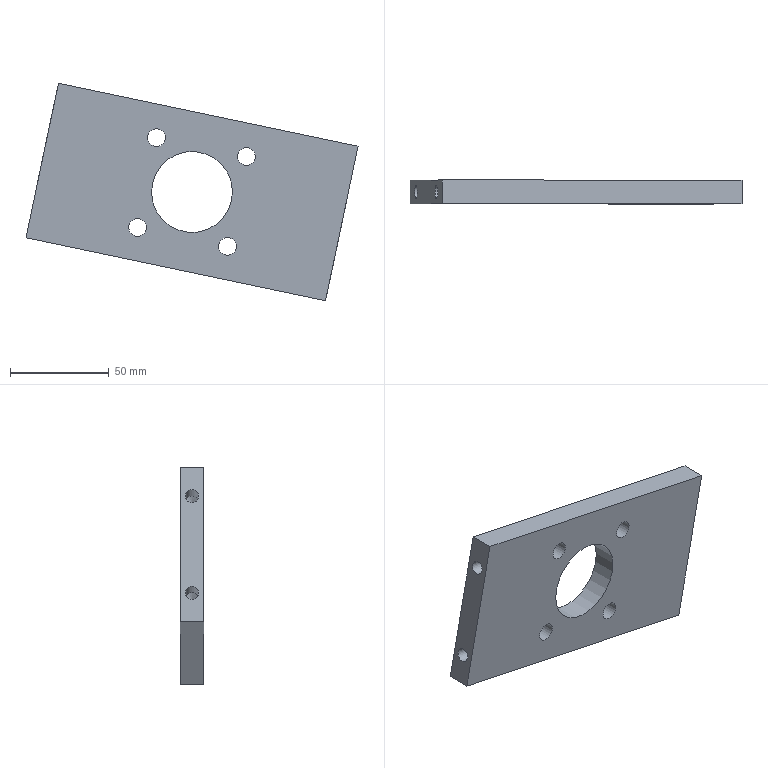Part | STEP file | SN10_007_005_PLACA | 1 solid | 19 faces | box 168.139 x 12 x 110.165 mm | volume 127729 mm3 | cylinder 9 | plane 6 | cone 4 | commonest cylinder face diameters 6.647 x4 9 x4 41 x1
STEP:
#1=CARTESIAN_POINT('',(0.,0.,0.));
#2=DIRECTION('',(0.,0.,1.));
#3=DIRECTION('',(1.,0.,0.));
#4=AXIS2_PLACEMENT_3D('',#1,#2,#3);
#5=CARTESIAN_POINT('',(-580.508,-921.15,530.345));
#6=VERTEX_POINT('',#5);
#7=CARTESIAN_POINT('',(-600.57,-921.15,534.561));
#8=DIRECTION('',(0.,1.,0.));
#9=DIRECTION('',(-0.9786,0.,0.2056));
#10=AXIS2_PLACEMENT_3D('',#7,#8,#9);
#11=CIRCLE('',#10,20.5);
#12=CARTESIAN_POINT('',(-600.57,-909.15,534.561));
#13=DIRECTION('',(0.,-1.,0.));
#14=DIRECTION('',(-0.9786,0.,0.2056));
#15=AXIS2_PLACEMENT_3D('',#12,#13,#14);
#16=CYLINDRICAL_SURFACE('',#15,20.5);
#17=CARTESIAN_POINT('',(12.566,12.));
#18=DIRECTION('',(-1.,0.));
#19=VECTOR('',#18,1.);
#20=LINE('',#17,#19);
#21=(GEOMETRIC_REPRESENTATION_CONTEXT(2)PARAMETRIC_REPRESENTATION_CONTEXT()REPRESENTATION_CONTEXT('',''));
#22=DEFINITIONAL_REPRESENTATION('',(#20),#21);
#23=PCURVE('',#16,#22);
#24=CARTESIAN_POINT('',(-537.207,-921.15,495.7));
#25=DIRECTION('',(0.,-1.,0.));
#26=DIRECTION('',(0.,0.,-1.));
#27=AXIS2_PLACEMENT_3D('',#24,#25,#26);
#28=PLANE('',#27);
#29=CARTESIAN_POINT('',(-43.076,-83.425));
#30=CARTESIAN_POINT('',(-77.825,-76.123));
#31=CARTESIAN_POINT('',(-54.127,-49.681));
#32=CARTESIAN_POINT('',(-30.429,-23.239));
#33=CARTESIAN_POINT('',(-19.379,-56.983));
#34=CARTESIAN_POINT('',(-8.328,-90.726));
#35=CARTESIAN_POINT('',(-43.076,-83.425));
#36=(BOUNDED_CURVE()B_SPLINE_CURVE(2,(#29,#30,#31,#32,#33,#34,#35),.UNSPECIFIED.,.T.,.F.)B_SPLINE_CURVE_WITH_KNOTS((1,2,2,2,2,1),(-2.094,0.,2.094,4.189,6.283,8.378),.UNSPECIFIED.)CURVE()GEOMETRIC_REPRESENTATION_ITEM()RATIONAL_B_SPLINE_CURVE((1.,0.5,1.,0.5,1.,0.5,1.))REPRESENTATION_ITEM(''));
#37=(GEOMETRIC_REPRESENTATION_CONTEXT(2)PARAMETRIC_REPRESENTATION_CONTEXT()REPRESENTATION_CONTEXT('',''));
#38=DEFINITIONAL_REPRESENTATION('',(#36),#37);
#39=PCURVE('',#28,#38);
#40=SURFACE_CURVE('',#11,(#23,#39),.PCURVE_S1.);
#41=EDGE_CURVE('',#6,#6,#40,.T.);
#42=ORIENTED_EDGE('',*,*,#41,.T.);
#43=CARTESIAN_POINT('',(-580.508,-909.15,530.345));
#44=VERTEX_POINT('',#43);
#45=CARTESIAN_POINT('',(-580.508,-909.15,530.345));
#46=CARTESIAN_POINT('',(-580.508,-921.15,530.345));
#47=B_SPLINE_CURVE_WITH_KNOTS('',1,(#45,#46),.UNSPECIFIED.,.F.,.F.,(2,2),(0.,12.),.PIECEWISE_BEZIER_KNOTS.);
#48=CARTESIAN_POINT('',(3.142,0.));
#49=DIRECTION('',(0.,1.));
#50=VECTOR('',#49,1.);
#51=LINE('',#48,#50);
#52=(GEOMETRIC_REPRESENTATION_CONTEXT(2)PARAMETRIC_REPRESENTATION_CONTEXT()REPRESENTATION_CONTEXT('',''));
#53=DEFINITIONAL_REPRESENTATION('',(#51),#52);
#54=PCURVE('',#16,#53);
#55=CARTESIAN_POINT('',(9.425,0.));
#56=DIRECTION('',(0.,1.));
#57=VECTOR('',#56,1.);
#58=LINE('',#55,#57);
#59=(GEOMETRIC_REPRESENTATION_CONTEXT(2)PARAMETRIC_REPRESENTATION_CONTEXT()REPRESENTATION_CONTEXT('',''));
#60=DEFINITIONAL_REPRESENTATION('',(#58),#59);
#61=PCURVE('',#16,#60);
#62=SEAM_CURVE('',#47,(#54,#61),.PCURVE_S1.);
#63=EDGE_CURVE('',#44,#6,#62,.T.);
#64=ORIENTED_EDGE('',*,*,#63,.F.);
#65=CARTESIAN_POINT('',(-600.57,-909.15,534.561));
#66=DIRECTION('',(0.,-1.,0.));
#67=DIRECTION('',(-0.9786,0.,0.2056));
#68=AXIS2_PLACEMENT_3D('',#65,#66,#67);
#69=CIRCLE('',#68,20.5);
#70=CARTESIAN_POINT('',(0.,0.));
#71=DIRECTION('',(1.,0.));
#72=VECTOR('',#71,1.);
#73=LINE('',#70,#72);
#74=(GEOMETRIC_REPRESENTATION_CONTEXT(2)PARAMETRIC_REPRESENTATION_CONTEXT()REPRESENTATION_CONTEXT('',''));
#75=DEFINITIONAL_REPRESENTATION('',(#73),#74);
#76=PCURVE('',#16,#75);
#77=CARTESIAN_POINT('',(0.,-909.15,0.));
#78=DIRECTION('',(0.,1.,0.));
#79=DIRECTION('',(0.,0.,1.));
#80=AXIS2_PLACEMENT_3D('',#77,#78,#79);
#81=PLANE('',#80);
#82=CARTESIAN_POINT('',(538.777,-620.632));
#83=CARTESIAN_POINT('',(504.029,-627.934));
#84=CARTESIAN_POINT('',(515.079,-594.19));
#85=CARTESIAN_POINT('',(526.13,-560.447));
#86=CARTESIAN_POINT('',(549.827,-586.888));
#87=CARTESIAN_POINT('',(573.525,-613.33));
#88=CARTESIAN_POINT('',(538.777,-620.632));
#89=(BOUNDED_CURVE()B_SPLINE_CURVE(2,(#82,#83,#84,#85,#86,#87,#88),.UNSPECIFIED.,.T.,.F.)B_SPLINE_CURVE_WITH_KNOTS((1,2,2,2,2,1),(-2.094,0.,2.094,4.189,6.283,8.378),.UNSPECIFIED.)CURVE()GEOMETRIC_REPRESENTATION_ITEM()RATIONAL_B_SPLINE_CURVE((1.,0.5,1.,0.5,1.,0.5,1.))REPRESENTATION_ITEM(''));
#90=(GEOMETRIC_REPRESENTATION_CONTEXT(2)PARAMETRIC_REPRESENTATION_CONTEXT()REPRESENTATION_CONTEXT('',''));
#91=DEFINITIONAL_REPRESENTATION('',(#89),#90);
#92=PCURVE('',#81,#91);
#93=SURFACE_CURVE('',#69,(#76,#92),.PCURVE_S1.);
#94=EDGE_CURVE('',#44,#44,#93,.T.);
#95=ORIENTED_EDGE('',*,*,#94,.T.);
#96=ORIENTED_EDGE('',*,*,#63,.T.);
#97=EDGE_LOOP('',(#42,#64,#95,#96));
#98=FACE_BOUND('',#97,.F.);
#99=ADVANCED_FACE('',(#98),#16,.F.);
#100=CARTESIAN_POINT('',(-545.231,-915.15,493.99));
#101=VERTEX_POINT('',#100);
#102=CARTESIAN_POINT('',(-544.547,-915.15,497.243));
#103=DIRECTION('',(0.9786,0.,-0.2056));
#104=DIRECTION('',(-0.2056,0.,-0.9786));
#105=AXIS2_PLACEMENT_3D('',#102,#103,#104);
#106=CIRCLE('',#105,3.324);
#107=CARTESIAN_POINT('',(-545.524,-915.15,497.448));
#108=DIRECTION('',(0.9786,0.,-0.2056));
#109=DIRECTION('',(-0.2056,0.,-0.9786));
#110=AXIS2_PLACEMENT_3D('',#107,#108,#109);
#111=CONICAL_SURFACE('',#110,1.662,1.03);
#112=CARTESIAN_POINT('',(0.,0.9985));
#113=DIRECTION('',(1.,0.));
#114=VECTOR('',#113,1.);
#115=LINE('',#112,#114);
#116=(GEOMETRIC_REPRESENTATION_CONTEXT(2)PARAMETRIC_REPRESENTATION_CONTEXT()REPRESENTATION_CONTEXT('',''));
#117=DEFINITIONAL_REPRESENTATION('',(#115),#116);
#118=PCURVE('',#111,#117);
#119=CARTESIAN_POINT('',(-537.207,-915.15,495.7));
#120=DIRECTION('',(0.9786,0.,-0.2056));
#121=DIRECTION('',(-0.2056,0.,-0.9786));
#122=AXIS2_PLACEMENT_3D('',#119,#120,#121);
#123=CYLINDRICAL_SURFACE('',#122,3.324);
#124=CARTESIAN_POINT('',(0.,-7.5));
#125=DIRECTION('',(1.,0.));
#126=VECTOR('',#125,1.);
#127=LINE('',#124,#126);
#128=(GEOMETRIC_REPRESENTATION_CONTEXT(2)PARAMETRIC_REPRESENTATION_CONTEXT()REPRESENTATION_CONTEXT('',''));
#129=DEFINITIONAL_REPRESENTATION('',(#127),#128);
#130=PCURVE('',#123,#129);
#131=SURFACE_CURVE('',#106,(#118,#130),.PCURVE_S1.);
#132=EDGE_CURVE('',#101,#101,#131,.T.);
#133=ORIENTED_EDGE('',*,*,#132,.F.);
#134=CARTESIAN_POINT('',(-546.501,-915.15,497.653));
#135=VERTEX_POINT('',#134);
#136=CARTESIAN_POINT('',(-546.501,-915.15,497.653));
#137=CARTESIAN_POINT('',(-545.231,-915.15,493.99));
#138=B_SPLINE_CURVE_WITH_KNOTS('',1,(#136,#137),.UNSPECIFIED.,.F.,.F.,(2,2),(-1.939,1.939),.PIECEWISE_BEZIER_KNOTS.);
#139=CARTESIAN_POINT('',(0.,0.));
#140=DIRECTION('',(0.,1.));
#141=VECTOR('',#140,1.);
#142=LINE('',#139,#141);
#143=(GEOMETRIC_REPRESENTATION_CONTEXT(2)PARAMETRIC_REPRESENTATION_CONTEXT()REPRESENTATION_CONTEXT('',''));
#144=DEFINITIONAL_REPRESENTATION('',(#142),#143);
#145=PCURVE('',#111,#144);
#146=CARTESIAN_POINT('',(6.283,0.));
#147=DIRECTION('',(0.,1.));
#148=VECTOR('',#147,1.);
#149=LINE('',#146,#148);
#150=(GEOMETRIC_REPRESENTATION_CONTEXT(2)PARAMETRIC_REPRESENTATION_CONTEXT()REPRESENTATION_CONTEXT('',''));
#151=DEFINITIONAL_REPRESENTATION('',(#149),#150);
#152=PCURVE('',#111,#151);
#153=SEAM_CURVE('',#138,(#145,#152),.PCURVE_S1.);
#154=EDGE_CURVE('',#135,#101,#153,.T.);
#155=ORIENTED_EDGE('',*,*,#154,.F.);
#156=ORIENTED_EDGE('',*,*,#154,.T.);
#157=EDGE_LOOP('',(#133,#155,#156));
#158=FACE_BOUND('',#157,.F.);
#159=ADVANCED_FACE('',(#158),#111,.F.);
#160=CARTESIAN_POINT('',(-530.551,-915.15,490.906));
#161=VERTEX_POINT('',#160);
#162=CARTESIAN_POINT('',(-529.868,-915.15,494.158));
#163=DIRECTION('',(-0.9786,0.,0.2056));
#164=DIRECTION('',(-0.2056,0.,-0.9786));
#165=AXIS2_PLACEMENT_3D('',#162,#163,#164);
#166=CIRCLE('',#165,3.324);
#167=CARTESIAN_POINT('',(6.283,7.5));
#168=DIRECTION('',(-1.,0.));
#169=VECTOR('',#168,1.);
#170=LINE('',#167,#169);
#171=(GEOMETRIC_REPRESENTATION_CONTEXT(2)PARAMETRIC_REPRESENTATION_CONTEXT()REPRESENTATION_CONTEXT('',''));
#172=DEFINITIONAL_REPRESENTATION('',(#170),#171);
#173=PCURVE('',#123,#172);
#174=CARTESIAN_POINT('',(-516.501,-909.15,557.769));
#175=DIRECTION('',(-0.9786,0.,0.2056));
#176=DIRECTION('',(0.2056,0.,0.9786));
#177=AXIS2_PLACEMENT_3D('',#174,#175,#176);
#178=PLANE('',#177);
#179=CARTESIAN_POINT('',(-65.,-6.));
#180=DIRECTION('',(-1.,0.));
#181=AXIS2_PLACEMENT_2D('',#179,#180);
#182=CIRCLE('',#181,3.324);
#183=(GEOMETRIC_REPRESENTATION_CONTEXT(2)PARAMETRIC_REPRESENTATION_CONTEXT()REPRESENTATION_CONTEXT('',''));
#184=DEFINITIONAL_REPRESENTATION('',(#182),#183);
#185=PCURVE('',#178,#184);
#186=SURFACE_CURVE('',#166,(#173,#185),.PCURVE_S1.);
#187=EDGE_CURVE('',#161,#161,#186,.T.);
#188=ORIENTED_EDGE('',*,*,#187,.T.);
#189=CARTESIAN_POINT('',(-545.231,-915.15,493.99));
#190=CARTESIAN_POINT('',(-530.551,-915.15,490.906));
#191=B_SPLINE_CURVE_WITH_KNOTS('',1,(#189,#190),.UNSPECIFIED.,.F.,.F.,(2,2),(-7.5,7.5),.PIECEWISE_BEZIER_KNOTS.);
#192=CARTESIAN_POINT('',(0.,0.));
#193=DIRECTION('',(0.,1.));
#194=VECTOR('',#193,1.);
#195=LINE('',#192,#194);
#196=(GEOMETRIC_REPRESENTATION_CONTEXT(2)PARAMETRIC_REPRESENTATION_CONTEXT()REPRESENTATION_CONTEXT('',''));
#197=DEFINITIONAL_REPRESENTATION('',(#195),#196);
#198=PCURVE('',#123,#197);
#199=CARTESIAN_POINT('',(6.283,0.));
#200=DIRECTION('',(0.,1.));
#201=VECTOR('',#200,1.);
#202=LINE('',#199,#201);
#203=(GEOMETRIC_REPRESENTATION_CONTEXT(2)PARAMETRIC_REPRESENTATION_CONTEXT()REPRESENTATION_CONTEXT('',''));
#204=DEFINITIONAL_REPRESENTATION('',(#202),#203);
#205=PCURVE('',#123,#204);
#206=SEAM_CURVE('',#191,(#198,#205),.PCURVE_S1.);
#207=EDGE_CURVE('',#101,#161,#206,.T.);
#208=ORIENTED_EDGE('',*,*,#207,.F.);
#209=ORIENTED_EDGE('',*,*,#132,.T.);
#210=ORIENTED_EDGE('',*,*,#207,.T.);
#211=EDGE_LOOP('',(#188,#208,#209,#210));
#212=FACE_BOUND('',#211,.F.);
#213=ADVANCED_FACE('',(#212),#123,.F.);
#214=CARTESIAN_POINT('',(-534.948,-915.15,542.922));
#215=VERTEX_POINT('',#214);
#216=CARTESIAN_POINT('',(-534.265,-915.15,546.174));
#217=DIRECTION('',(0.9786,0.,-0.2056));
#218=DIRECTION('',(-0.2056,0.,-0.9786));
#219=AXIS2_PLACEMENT_3D('',#216,#217,#218);
#220=CIRCLE('',#219,3.324);
#221=CARTESIAN_POINT('',(-535.242,-915.15,546.379));
#222=DIRECTION('',(0.9786,0.,-0.2056));
#223=DIRECTION('',(-0.2056,0.,-0.9786));
#224=AXIS2_PLACEMENT_3D('',#221,#222,#223);
#225=CONICAL_SURFACE('',#224,1.662,1.03);
#226=CARTESIAN_POINT('',(0.,0.9985));
#227=DIRECTION('',(1.,0.));
#228=VECTOR('',#227,1.);
#229=LINE('',#226,#228);
#230=(GEOMETRIC_REPRESENTATION_CONTEXT(2)PARAMETRIC_REPRESENTATION_CONTEXT()REPRESENTATION_CONTEXT('',''));
#231=DEFINITIONAL_REPRESENTATION('',(#229),#230);
#232=PCURVE('',#225,#231);
#233=CARTESIAN_POINT('',(-526.925,-915.15,544.632));
#234=DIRECTION('',(0.9786,0.,-0.2056));
#235=DIRECTION('',(-0.2056,0.,-0.9786));
#236=AXIS2_PLACEMENT_3D('',#233,#234,#235);
#237=CYLINDRICAL_SURFACE('',#236,3.324);
#238=CARTESIAN_POINT('',(0.,-7.5));
#239=DIRECTION('',(1.,0.));
#240=VECTOR('',#239,1.);
#241=LINE('',#238,#240);
#242=(GEOMETRIC_REPRESENTATION_CONTEXT(2)PARAMETRIC_REPRESENTATION_CONTEXT()REPRESENTATION_CONTEXT('',''));
#243=DEFINITIONAL_REPRESENTATION('',(#241),#242);
#244=PCURVE('',#237,#243);
#245=SURFACE_CURVE('',#220,(#232,#244),.PCURVE_S1.);
#246=EDGE_CURVE('',#215,#215,#245,.T.);
#247=ORIENTED_EDGE('',*,*,#246,.F.);
#248=CARTESIAN_POINT('',(-536.219,-915.15,546.585));
#249=VERTEX_POINT('',#248);
#250=CARTESIAN_POINT('',(-536.219,-915.15,546.585));
#251=CARTESIAN_POINT('',(-534.948,-915.15,542.922));
#252=B_SPLINE_CURVE_WITH_KNOTS('',1,(#250,#251),.UNSPECIFIED.,.F.,.F.,(2,2),(-1.939,1.939),.PIECEWISE_BEZIER_KNOTS.);
#253=CARTESIAN_POINT('',(0.,0.));
#254=DIRECTION('',(0.,1.));
#255=VECTOR('',#254,1.);
#256=LINE('',#253,#255);
#257=(GEOMETRIC_REPRESENTATION_CONTEXT(2)PARAMETRIC_REPRESENTATION_CONTEXT()REPRESENTATION_CONTEXT('',''));
#258=DEFINITIONAL_REPRESENTATION('',(#256),#257);
#259=PCURVE('',#225,#258);
#260=CARTESIAN_POINT('',(6.283,0.));
#261=DIRECTION('',(0.,1.));
#262=VECTOR('',#261,1.);
#263=LINE('',#260,#262);
#264=(GEOMETRIC_REPRESENTATION_CONTEXT(2)PARAMETRIC_REPRESENTATION_CONTEXT()REPRESENTATION_CONTEXT('',''));
#265=DEFINITIONAL_REPRESENTATION('',(#263),#264);
#266=PCURVE('',#225,#265);
#267=SEAM_CURVE('',#252,(#259,#266),.PCURVE_S1.);
#268=EDGE_CURVE('',#249,#215,#267,.T.);
#269=ORIENTED_EDGE('',*,*,#268,.F.);
#270=ORIENTED_EDGE('',*,*,#268,.T.);
#271=EDGE_LOOP('',(#247,#269,#270));
#272=FACE_BOUND('',#271,.F.);
#273=ADVANCED_FACE('',(#272),#225,.F.);
#274=CARTESIAN_POINT('',(-520.269,-915.15,539.837));
#275=VERTEX_POINT('',#274);
#276=CARTESIAN_POINT('',(-519.586,-915.15,543.089));
#277=DIRECTION('',(-0.9786,0.,0.2056));
#278=DIRECTION('',(-0.2056,0.,-0.9786));
#279=AXIS2_PLACEMENT_3D('',#276,#277,#278);
#280=CIRCLE('',#279,3.324);
#281=CARTESIAN_POINT('',(6.283,7.5));
#282=DIRECTION('',(-1.,0.));
#283=VECTOR('',#282,1.);
#284=LINE('',#281,#283);
#285=(GEOMETRIC_REPRESENTATION_CONTEXT(2)PARAMETRIC_REPRESENTATION_CONTEXT()REPRESENTATION_CONTEXT('',''));
#286=DEFINITIONAL_REPRESENTATION('',(#284),#285);
#287=PCURVE('',#237,#286);
#288=CARTESIAN_POINT('',(-15.,-6.));
#289=DIRECTION('',(-1.,0.));
#290=AXIS2_PLACEMENT_2D('',#288,#289);
#291=CIRCLE('',#290,3.324);
#292=(GEOMETRIC_REPRESENTATION_CONTEXT(2)PARAMETRIC_REPRESENTATION_CONTEXT()REPRESENTATION_CONTEXT('',''));
#293=DEFINITIONAL_REPRESENTATION('',(#291),#292);
#294=PCURVE('',#178,#293);
#295=SURFACE_CURVE('',#280,(#287,#294),.PCURVE_S1.);
#296=EDGE_CURVE('',#275,#275,#295,.T.);
#297=ORIENTED_EDGE('',*,*,#296,.T.);
#298=CARTESIAN_POINT('',(-534.948,-915.15,542.922));
#299=CARTESIAN_POINT('',(-520.269,-915.15,539.837));
#300=B_SPLINE_CURVE_WITH_KNOTS('',1,(#298,#299),.UNSPECIFIED.,.F.,.F.,(2,2),(-7.5,7.5),.PIECEWISE_BEZIER_KNOTS.);
#301=CARTESIAN_POINT('',(0.,0.));
#302=DIRECTION('',(0.,1.));
#303=VECTOR('',#302,1.);
#304=LINE('',#301,#303);
#305=(GEOMETRIC_REPRESENTATION_CONTEXT(2)PARAMETRIC_REPRESENTATION_CONTEXT()REPRESENTATION_CONTEXT('',''));
#306=DEFINITIONAL_REPRESENTATION('',(#304),#305);
#307=PCURVE('',#237,#306);
#308=CARTESIAN_POINT('',(6.283,0.));
#309=DIRECTION('',(0.,1.));
#310=VECTOR('',#309,1.);
#311=LINE('',#308,#310);
#312=(GEOMETRIC_REPRESENTATION_CONTEXT(2)PARAMETRIC_REPRESENTATION_CONTEXT()REPRESENTATION_CONTEXT('',''));
#313=DEFINITIONAL_REPRESENTATION('',(#311),#312);
#314=PCURVE('',#237,#313);
#315=SEAM_CURVE('',#300,(#307,#314),.PCURVE_S1.);
#316=EDGE_CURVE('',#215,#275,#315,.T.);
#317=ORIENTED_EDGE('',*,*,#316,.F.);
#318=ORIENTED_EDGE('',*,*,#246,.T.);
#319=ORIENTED_EDGE('',*,*,#316,.T.);
#320=EDGE_LOOP('',(#297,#317,#318,#319));
#321=FACE_BOUND('',#320,.F.);
#322=ADVANCED_FACE('',(#321),#237,.F.);
#323=CARTESIAN_POINT('',(-655.91,-915.15,575.132));
#324=VERTEX_POINT('',#323);
#325=CARTESIAN_POINT('',(-656.593,-915.15,571.88));
#326=DIRECTION('',(-0.9786,0.,0.2056));
#327=DIRECTION('',(0.2056,0.,0.9786));
#328=AXIS2_PLACEMENT_3D('',#325,#326,#327);
#329=CIRCLE('',#328,3.324);
#330=CARTESIAN_POINT('',(-655.616,-915.15,571.674));
#331=DIRECTION('',(-0.9786,0.,0.2056));
#332=DIRECTION('',(0.2056,0.,0.9786));
#333=AXIS2_PLACEMENT_3D('',#330,#331,#332);
#334=CONICAL_SURFACE('',#333,1.662,1.03);
#335=CARTESIAN_POINT('',(0.,0.9985));
#336=DIRECTION('',(1.,0.));
#337=VECTOR('',#336,1.);
#338=LINE('',#335,#337);
#339=(GEOMETRIC_REPRESENTATION_CONTEXT(2)PARAMETRIC_REPRESENTATION_CONTEXT()REPRESENTATION_CONTEXT('',''));
#340=DEFINITIONAL_REPRESENTATION('',(#338),#339);
#341=PCURVE('',#334,#340);
#342=CARTESIAN_POINT('',(-663.933,-915.15,573.422));
#343=DIRECTION('',(-0.9786,0.,0.2056));
#344=DIRECTION('',(0.2056,0.,0.9786));
#345=AXIS2_PLACEMENT_3D('',#342,#343,#344);
#346=CYLINDRICAL_SURFACE('',#345,3.324);
#347=CARTESIAN_POINT('',(0.,-7.5));
#348=DIRECTION('',(1.,0.));
#349=VECTOR('',#348,1.);
#350=LINE('',#347,#349);
#351=(GEOMETRIC_REPRESENTATION_CONTEXT(2)PARAMETRIC_REPRESENTATION_CONTEXT()REPRESENTATION_CONTEXT('',''));
#352=DEFINITIONAL_REPRESENTATION('',(#350),#351);
#353=PCURVE('',#346,#352);
#354=SURFACE_CURVE('',#329,(#341,#353),.PCURVE_S1.);
#355=EDGE_CURVE('',#324,#324,#354,.T.);
#356=ORIENTED_EDGE('',*,*,#355,.F.);
#357=CARTESIAN_POINT('',(-654.639,-915.15,571.469));
#358=VERTEX_POINT('',#357);
#359=CARTESIAN_POINT('',(-654.639,-915.15,571.469));
#360=CARTESIAN_POINT('',(-655.91,-915.15,575.132));
#361=B_SPLINE_CURVE_WITH_KNOTS('',1,(#359,#360),.UNSPECIFIED.,.F.,.F.,(2,2),(-1.939,1.939),.PIECEWISE_BEZIER_KNOTS.);
#362=CARTESIAN_POINT('',(0.,0.));
#363=DIRECTION('',(0.,1.));
#364=VECTOR('',#363,1.);
#365=LINE('',#362,#364);
#366=(GEOMETRIC_REPRESENTATION_CONTEXT(2)PARAMETRIC_REPRESENTATION_CONTEXT()REPRESENTATION_CONTEXT('',''));
#367=DEFINITIONAL_REPRESENTATION('',(#365),#366);
#368=PCURVE('',#334,#367);
#369=CARTESIAN_POINT('',(6.283,0.));
#370=DIRECTION('',(0.,1.));
#371=VECTOR('',#370,1.);
#372=LINE('',#369,#371);
#373=(GEOMETRIC_REPRESENTATION_CONTEXT(2)PARAMETRIC_REPRESENTATION_CONTEXT()REPRESENTATION_CONTEXT('',''));
#374=DEFINITIONAL_REPRESENTATION('',(#372),#373);
#375=PCURVE('',#334,#374);
#376=SEAM_CURVE('',#361,(#368,#375),.PCURVE_S1.);
#377=EDGE_CURVE('',#358,#324,#376,.T.);
#378=ORIENTED_EDGE('',*,*,#377,.F.);
#379=ORIENTED_EDGE('',*,*,#377,.T.);
#380=EDGE_LOOP('',(#356,#378,#379));
#381=FACE_BOUND('',#380,.F.);
#382=ADVANCED_FACE('',(#381),#334,.F.);
#383=CARTESIAN_POINT('',(-670.589,-915.15,578.217));
#384=VERTEX_POINT('',#383);
#385=CARTESIAN_POINT('',(-671.273,-915.15,574.964));
#386=DIRECTION('',(0.9786,0.,-0.2056));
#387=DIRECTION('',(0.2056,0.,0.9786));
#388=AXIS2_PLACEMENT_3D('',#385,#386,#387);
#389=CIRCLE('',#388,3.324);
#390=CARTESIAN_POINT('',(6.283,7.5));
#391=DIRECTION('',(-1.,0.));
#392=VECTOR('',#391,1.);
#393=LINE('',#390,#392);
#394=(GEOMETRIC_REPRESENTATION_CONTEXT(2)PARAMETRIC_REPRESENTATION_CONTEXT()REPRESENTATION_CONTEXT('',''));
#395=DEFINITIONAL_REPRESENTATION('',(#393),#394);
#396=PCURVE('',#346,#395);
#397=CARTESIAN_POINT('',(-668.188,-921.15,589.644));
#398=DIRECTION('',(0.9786,0.,-0.2056));
#399=DIRECTION('',(-0.2056,0.,-0.9786));
#400=AXIS2_PLACEMENT_3D('',#397,#398,#399);
#401=PLANE('',#400);
#402=CARTESIAN_POINT('',(15.,6.));
#403=DIRECTION('',(-1.,0.));
#404=AXIS2_PLACEMENT_2D('',#402,#403);
#405=CIRCLE('',#404,3.324);
#406=(GEOMETRIC_REPRESENTATION_CONTEXT(2)PARAMETRIC_REPRESENTATION_CONTEXT()REPRESENTATION_CONTEXT('',''));
#407=DEFINITIONAL_REPRESENTATION('',(#405),#406);
#408=PCURVE('',#401,#407);
#409=SURFACE_CURVE('',#389,(#396,#408),.PCURVE_S1.);
#410=EDGE_CURVE('',#384,#384,#409,.T.);
#411=ORIENTED_EDGE('',*,*,#410,.T.);
#412=CARTESIAN_POINT('',(-655.91,-915.15,575.132));
#413=CARTESIAN_POINT('',(-670.589,-915.15,578.217));
#414=B_SPLINE_CURVE_WITH_KNOTS('',1,(#412,#413),.UNSPECIFIED.,.F.,.F.,(2,2),(-7.5,7.5),.PIECEWISE_BEZIER_KNOTS.);
#415=CARTESIAN_POINT('',(0.,0.));
#416=DIRECTION('',(0.,1.));
#417=VECTOR('',#416,1.);
#418=LINE('',#415,#417);
#419=(GEOMETRIC_REPRESENTATION_CONTEXT(2)PARAMETRIC_REPRESENTATION_CONTEXT()REPRESENTATION_CONTEXT('',''));
#420=DEFINITIONAL_REPRESENTATION('',(#418),#419);
#421=PCURVE('',#346,#420);
#422=CARTESIAN_POINT('',(6.283,0.));
#423=DIRECTION('',(0.,1.));
#424=VECTOR('',#423,1.);
#425=LINE('',#422,#424);
#426=(GEOMETRIC_REPRESENTATION_CONTEXT(2)PARAMETRIC_REPRESENTATION_CONTEXT()REPRESENTATION_CONTEXT('',''));
#427=DEFINITIONAL_REPRESENTATION('',(#425),#426);
#428=PCURVE('',#346,#427);
#429=SEAM_CURVE('',#414,(#421,#428),.PCURVE_S1.);
#430=EDGE_CURVE('',#324,#384,#429,.T.);
#431=ORIENTED_EDGE('',*,*,#430,.F.);
#432=ORIENTED_EDGE('',*,*,#355,.T.);
#433=ORIENTED_EDGE('',*,*,#430,.T.);
#434=EDGE_LOOP('',(#411,#431,#432,#433));
#435=FACE_BOUND('',#434,.F.);
#436=ADVANCED_FACE('',(#435),#346,.F.);
#437=CARTESIAN_POINT('',(-666.192,-915.15,526.201));
#438=VERTEX_POINT('',#437);
#439=CARTESIAN_POINT('',(-666.875,-915.15,522.948));
#440=DIRECTION('',(-0.9786,0.,0.2056));
#441=DIRECTION('',(0.2056,0.,0.9786));
#442=AXIS2_PLACEMENT_3D('',#439,#440,#441);
#443=CIRCLE('',#442,3.324);
#444=CARTESIAN_POINT('',(-665.898,-915.15,522.743));
#445=DIRECTION('',(-0.9786,0.,0.2056));
#446=DIRECTION('',(0.2056,0.,0.9786));
#447=AXIS2_PLACEMENT_3D('',#444,#445,#446);
#448=CONICAL_SURFACE('',#447,1.662,1.03);
#449=CARTESIAN_POINT('',(0.,0.9985));
#450=DIRECTION('',(1.,0.));
#451=VECTOR('',#450,1.);
#452=LINE('',#449,#451);
#453=(GEOMETRIC_REPRESENTATION_CONTEXT(2)PARAMETRIC_REPRESENTATION_CONTEXT()REPRESENTATION_CONTEXT('',''));
#454=DEFINITIONAL_REPRESENTATION('',(#452),#453);
#455=PCURVE('',#448,#454);
#456=CARTESIAN_POINT('',(-674.215,-915.15,524.49));
#457=DIRECTION('',(-0.9786,0.,0.2056));
#458=DIRECTION('',(0.2056,0.,0.9786));
#459=AXIS2_PLACEMENT_3D('',#456,#457,#458);
#460=CYLINDRICAL_SURFACE('',#459,3.324);
#461=CARTESIAN_POINT('',(0.,-7.5));
#462=DIRECTION('',(1.,0.));
#463=VECTOR('',#462,1.);
#464=LINE('',#461,#463);
#465=(GEOMETRIC_REPRESENTATION_CONTEXT(2)PARAMETRIC_REPRESENTATION_CONTEXT()REPRESENTATION_CONTEXT('',''));
#466=DEFINITIONAL_REPRESENTATION('',(#464),#465);
#467=PCURVE('',#460,#466);
#468=SURFACE_CURVE('',#443,(#455,#467),.PCURVE_S1.);
#469=EDGE_CURVE('',#438,#438,#468,.T.);
#470=ORIENTED_EDGE('',*,*,#469,.F.);
#471=CARTESIAN_POINT('',(-664.921,-915.15,522.537));
#472=VERTEX_POINT('',#471);
#473=CARTESIAN_POINT('',(-664.921,-915.15,522.537));
#474=CARTESIAN_POINT('',(-666.192,-915.15,526.201));
#475=B_SPLINE_CURVE_WITH_KNOTS('',1,(#473,#474),.UNSPECIFIED.,.F.,.F.,(2,2),(-1.939,1.939),.PIECEWISE_BEZIER_KNOTS.);
#476=CARTESIAN_POINT('',(0.,0.));
#477=DIRECTION('',(0.,1.));
#478=VECTOR('',#477,1.);
#479=LINE('',#476,#478);
#480=(GEOMETRIC_REPRESENTATION_CONTEXT(2)PARAMETRIC_REPRESENTATION_CONTEXT()REPRESENTATION_CONTEXT('',''));
#481=DEFINITIONAL_REPRESENTATION('',(#479),#480);
#482=PCURVE('',#448,#481);
#483=CARTESIAN_POINT('',(6.283,0.));
#484=DIRECTION('',(0.,1.));
#485=VECTOR('',#484,1.);
#486=LINE('',#483,#485);
#487=(GEOMETRIC_REPRESENTATION_CONTEXT(2)PARAMETRIC_REPRESENTATION_CONTEXT()REPRESENTATION_CONTEXT('',''));
#488=DEFINITIONAL_REPRESENTATION('',(#486),#487);
#489=PCURVE('',#448,#488);
#490=SEAM_CURVE('',#475,(#482,#489),.PCURVE_S1.);
#491=EDGE_CURVE('',#472,#438,#490,.T.);
#492=ORIENTED_EDGE('',*,*,#491,.F.);
#493=ORIENTED_EDGE('',*,*,#491,.T.);
#494=EDGE_LOOP('',(#470,#492,#493));
#495=FACE_BOUND('',#494,.F.);
#496=ADVANCED_FACE('',(#495),#448,.F.);
#497=CARTESIAN_POINT('',(-680.871,-915.15,529.285));
#498=VERTEX_POINT('',#497);
#499=CARTESIAN_POINT('',(-681.555,-915.15,526.033));
#500=DIRECTION('',(0.9786,0.,-0.2056));
#501=DIRECTION('',(0.2056,0.,0.9786));
#502=AXIS2_PLACEMENT_3D('',#499,#500,#501);
#503=CIRCLE('',#502,3.324);
#504=CARTESIAN_POINT('',(6.283,7.5));
#505=DIRECTION('',(-1.,0.));
#506=VECTOR('',#505,1.);
#507=LINE('',#504,#506);
#508=(GEOMETRIC_REPRESENTATION_CONTEXT(2)PARAMETRIC_REPRESENTATION_CONTEXT()REPRESENTATION_CONTEXT('',''));
#509=DEFINITIONAL_REPRESENTATION('',(#507),#508);
#510=PCURVE('',#460,#509);
#511=CARTESIAN_POINT('',(65.,6.));
#512=DIRECTION('',(-1.,0.));
#513=AXIS2_PLACEMENT_2D('',#511,#512);
#514=CIRCLE('',#513,3.324);
#515=(GEOMETRIC_REPRESENTATION_CONTEXT(2)PARAMETRIC_REPRESENTATION_CONTEXT()REPRESENTATION_CONTEXT('',''));
#516=DEFINITIONAL_REPRESENTATION('',(#514),#515);
#517=PCURVE('',#401,#516);
#518=SURFACE_CURVE('',#503,(#510,#517),.PCURVE_S1.);
#519=EDGE_CURVE('',#498,#498,#518,.T.);
#520=ORIENTED_EDGE('',*,*,#519,.T.);
#521=CARTESIAN_POINT('',(-666.192,-915.15,526.201));
#522=CARTESIAN_POINT('',(-680.871,-915.15,529.285));
#523=B_SPLINE_CURVE_WITH_KNOTS('',1,(#521,#522),.UNSPECIFIED.,.F.,.F.,(2,2),(-7.5,7.5),.PIECEWISE_BEZIER_KNOTS.);
#524=CARTESIAN_POINT('',(0.,0.));
#525=DIRECTION('',(0.,1.));
#526=VECTOR('',#525,1.);
#527=LINE('',#524,#526);
#528=(GEOMETRIC_REPRESENTATION_CONTEXT(2)PARAMETRIC_REPRESENTATION_CONTEXT()REPRESENTATION_CONTEXT('',''));
#529=DEFINITIONAL_REPRESENTATION('',(#527),#528);
#530=PCURVE('',#460,#529);
#531=CARTESIAN_POINT('',(6.283,0.));
#532=DIRECTION('',(0.,1.));
#533=VECTOR('',#532,1.);
#534=LINE('',#531,#533);
#535=(GEOMETRIC_REPRESENTATION_CONTEXT(2)PARAMETRIC_REPRESENTATION_CONTEXT()REPRESENTATION_CONTEXT('',''));
#536=DEFINITIONAL_REPRESENTATION('',(#534),#535);
#537=PCURVE('',#460,#536);
#538=SEAM_CURVE('',#523,(#530,#537),.PCURVE_S1.);
#539=EDGE_CURVE('',#438,#498,#538,.T.);
#540=ORIENTED_EDGE('',*,*,#539,.F.);
#541=ORIENTED_EDGE('',*,*,#469,.T.);
#542=ORIENTED_EDGE('',*,*,#539,.T.);
#543=EDGE_LOOP('',(#520,#540,#541,#542));
#544=FACE_BOUND('',#543,.F.);
#545=ADVANCED_FACE('',(#544),#460,.F.);
#546=CARTESIAN_POINT('',(-532.952,-909.15,479.479));
#547=VERTEX_POINT('',#546);
#548=CARTESIAN_POINT('',(-532.952,-921.15,479.479));
#549=VERTEX_POINT('',#548);
#550=CARTESIAN_POINT('',(-532.952,-909.15,479.479));
#551=DIRECTION('',(0.,-1.,0.));
#552=VECTOR('',#551,1.);
#553=LINE('',#550,#552);
#554=CARTESIAN_POINT('',(-80.,0.));
#555=DIRECTION('',(0.,-1.));
#556=VECTOR('',#555,1.);
#557=LINE('',#554,#556);
#558=(GEOMETRIC_REPRESENTATION_CONTEXT(2)PARAMETRIC_REPRESENTATION_CONTEXT()REPRESENTATION_CONTEXT('',''));
#559=DEFINITIONAL_REPRESENTATION('',(#557),#558);
#560=PCURVE('',#178,#559);
#561=CARTESIAN_POINT('',(-687.086,-909.15,511.868));
#562=DIRECTION('',(-0.2056,0.,-0.9786));
#563=DIRECTION('',(-0.9786,0.,0.2056));
#564=AXIS2_PLACEMENT_3D('',#561,#562,#563);
#565=PLANE('',#564);
#566=CARTESIAN_POINT('',(-157.5,0.));
#567=DIRECTION('',(0.,-1.));
#568=VECTOR('',#567,1.);
#569=LINE('',#566,#568);
#570=(GEOMETRIC_REPRESENTATION_CONTEXT(2)PARAMETRIC_REPRESENTATION_CONTEXT()REPRESENTATION_CONTEXT('',''));
#571=DEFINITIONAL_REPRESENTATION('',(#569),#570);
#572=PCURVE('',#565,#571);
#573=SURFACE_CURVE('',#553,(#560,#572),.PCURVE_S1.);
#574=EDGE_CURVE('',#547,#549,#573,.T.);
#575=ORIENTED_EDGE('',*,*,#574,.F.);
#576=CARTESIAN_POINT('',(-516.501,-909.15,557.769));
#577=VERTEX_POINT('',#576);
#578=CARTESIAN_POINT('',(-516.501,-909.15,557.769));
#579=DIRECTION('',(-0.2056,0.,-0.9786));
#580=VECTOR('',#579,1.);
#581=LINE('',#578,#580);
#582=CARTESIAN_POINT('',(0.,0.));
#583=DIRECTION('',(-1.,0.));
#584=VECTOR('',#583,1.);
#585=LINE('',#582,#584);
#586=(GEOMETRIC_REPRESENTATION_CONTEXT(2)PARAMETRIC_REPRESENTATION_CONTEXT()REPRESENTATION_CONTEXT('',''));
#587=DEFINITIONAL_REPRESENTATION('',(#585),#586);
#588=PCURVE('',#178,#587);
#589=CARTESIAN_POINT('',(557.769,-516.501));
#590=DIRECTION('',(-0.9786,-0.2056));
#591=VECTOR('',#590,1.);
#592=LINE('',#589,#591);
#593=(GEOMETRIC_REPRESENTATION_CONTEXT(2)PARAMETRIC_REPRESENTATION_CONTEXT()REPRESENTATION_CONTEXT('',''));
#594=DEFINITIONAL_REPRESENTATION('',(#592),#593);
#595=PCURVE('',#81,#594);
#596=SURFACE_CURVE('',#581,(#588,#595),.PCURVE_S1.);
#597=EDGE_CURVE('',#577,#547,#596,.T.);
#598=ORIENTED_EDGE('',*,*,#597,.F.);
#599=CARTESIAN_POINT('',(-516.501,-921.15,557.769));
#600=VERTEX_POINT('',#599);
#601=CARTESIAN_POINT('',(-516.501,-921.15,557.769));
#602=DIRECTION('',(0.,1.,0.));
#603=VECTOR('',#602,1.);
#604=LINE('',#601,#603);
#605=CARTESIAN_POINT('',(0.,-12.));
#606=DIRECTION('',(0.,1.));
#607=VECTOR('',#606,1.);
#608=LINE('',#605,#607);
#609=(GEOMETRIC_REPRESENTATION_CONTEXT(2)PARAMETRIC_REPRESENTATION_CONTEXT()REPRESENTATION_CONTEXT('',''));
#610=DEFINITIONAL_REPRESENTATION('',(#608),#609);
#611=PCURVE('',#178,#610);
#612=CARTESIAN_POINT('',(-514.054,-909.15,557.255));
#613=DIRECTION('',(0.2056,0.,0.9786));
#614=DIRECTION('',(0.9786,0.,-0.2056));
#615=AXIS2_PLACEMENT_3D('',#612,#613,#614);
#616=PLANE('',#615);
#617=CARTESIAN_POINT('',(-2.5,-12.));
#618=DIRECTION('',(0.,1.));
#619=VECTOR('',#618,1.);
#620=LINE('',#617,#619);
#621=(GEOMETRIC_REPRESENTATION_CONTEXT(2)PARAMETRIC_REPRESENTATION_CONTEXT()REPRESENTATION_CONTEXT('',''));
#622=DEFINITIONAL_REPRESENTATION('',(#620),#621);
#623=PCURVE('',#616,#622);
#624=SURFACE_CURVE('',#604,(#611,#623),.PCURVE_S1.);
#625=EDGE_CURVE('',#600,#577,#624,.T.);
#626=ORIENTED_EDGE('',*,*,#625,.F.);
#627=CARTESIAN_POINT('',(-532.952,-921.15,479.479));
#628=DIRECTION('',(0.2056,0.,0.9786));
#629=VECTOR('',#628,1.);
#630=LINE('',#627,#629);
#631=CARTESIAN_POINT('',(-80.,-12.));
#632=DIRECTION('',(1.,0.));
#633=VECTOR('',#632,1.);
#634=LINE('',#631,#633);
#635=(GEOMETRIC_REPRESENTATION_CONTEXT(2)PARAMETRIC_REPRESENTATION_CONTEXT()REPRESENTATION_CONTEXT('',''));
#636=DEFINITIONAL_REPRESENTATION('',(#634),#635);
#637=PCURVE('',#178,#636);
#638=CARTESIAN_POINT('',(16.222,4.255));
#639=DIRECTION('',(-0.9786,0.2056));
#640=VECTOR('',#639,1.);
#641=LINE('',#638,#640);
#642=(GEOMETRIC_REPRESENTATION_CONTEXT(2)PARAMETRIC_REPRESENTATION_CONTEXT()REPRESENTATION_CONTEXT('',''));
#643=DEFINITIONAL_REPRESENTATION('',(#641),#642);
#644=PCURVE('',#28,#643);
#645=SURFACE_CURVE('',#630,(#637,#644),.PCURVE_S1.);
#646=EDGE_CURVE('',#549,#600,#645,.T.);
#647=ORIENTED_EDGE('',*,*,#646,.F.);
#648=EDGE_LOOP('',(#575,#598,#626,#647));
#649=FACE_BOUND('',#648,.T.);
#650=ORIENTED_EDGE('',*,*,#187,.T.);
#651=EDGE_LOOP('',(#650));
#652=FACE_BOUND('',#651,.T.);
#653=ORIENTED_EDGE('',*,*,#296,.T.);
#654=EDGE_LOOP('',(#653));
#655=FACE_BOUND('',#654,.T.);
#656=ADVANCED_FACE('',(#649,#652,#655),#178,.F.);
#657=CARTESIAN_POINT('',(-684.64,-921.15,511.353));
#658=VERTEX_POINT('',#657);
#659=CARTESIAN_POINT('',(-684.64,-909.15,511.353));
#660=VERTEX_POINT('',#659);
#661=CARTESIAN_POINT('',(-684.64,-921.15,511.353));
#662=DIRECTION('',(0.,1.,0.));
#663=VECTOR('',#662,1.);
#664=LINE('',#661,#663);
#665=CARTESIAN_POINT('',(80.,0.));
#666=DIRECTION('',(0.,1.));
#667=VECTOR('',#666,1.);
#668=LINE('',#665,#667);
#669=(GEOMETRIC_REPRESENTATION_CONTEXT(2)PARAMETRIC_REPRESENTATION_CONTEXT()REPRESENTATION_CONTEXT('',''));
#670=DEFINITIONAL_REPRESENTATION('',(#668),#669);
#671=PCURVE('',#401,#670);
#672=CARTESIAN_POINT('',(-2.5,-12.));
#673=DIRECTION('',(0.,1.));
#674=VECTOR('',#673,1.);
#675=LINE('',#672,#674);
#676=(GEOMETRIC_REPRESENTATION_CONTEXT(2)PARAMETRIC_REPRESENTATION_CONTEXT()REPRESENTATION_CONTEXT('',''));
#677=DEFINITIONAL_REPRESENTATION('',(#675),#676);
#678=PCURVE('',#565,#677);
#679=SURFACE_CURVE('',#664,(#671,#678),.PCURVE_S1.);
#680=EDGE_CURVE('',#658,#660,#679,.T.);
#681=ORIENTED_EDGE('',*,*,#680,.F.);
#682=CARTESIAN_POINT('',(-668.188,-921.15,589.644));
#683=VERTEX_POINT('',#682);
#684=CARTESIAN_POINT('',(-668.188,-921.15,589.644));
#685=DIRECTION('',(-0.2056,0.,-0.9786));
#686=VECTOR('',#685,1.);
#687=LINE('',#684,#686);
#688=CARTESIAN_POINT('',(0.,0.));
#689=DIRECTION('',(1.,0.));
#690=VECTOR('',#689,1.);
#691=LINE('',#688,#690);
#692=(GEOMETRIC_REPRESENTATION_CONTEXT(2)PARAMETRIC_REPRESENTATION_CONTEXT()REPRESENTATION_CONTEXT('',''));
#693=DEFINITIONAL_REPRESENTATION('',(#691),#692);
#694=PCURVE('',#401,#693);
#695=CARTESIAN_POINT('',(-93.943,-130.981));
#696=DIRECTION('',(0.9786,-0.2056));
#697=VECTOR('',#696,1.);
#698=LINE('',#695,#697);
#699=(GEOMETRIC_REPRESENTATION_CONTEXT(2)PARAMETRIC_REPRESENTATION_CONTEXT()REPRESENTATION_CONTEXT('',''));
#700=DEFINITIONAL_REPRESENTATION('',(#698),#699);
#701=PCURVE('',#28,#700);
#702=SURFACE_CURVE('',#687,(#694,#701),.PCURVE_S1.);
#703=EDGE_CURVE('',#683,#658,#702,.T.);
#704=ORIENTED_EDGE('',*,*,#703,.F.);
#705=CARTESIAN_POINT('',(-668.188,-909.15,589.644));
#706=VERTEX_POINT('',#705);
#707=CARTESIAN_POINT('',(-668.188,-909.15,589.644));
#708=DIRECTION('',(0.,-1.,0.));
#709=VECTOR('',#708,1.);
#710=LINE('',#707,#709);
#711=CARTESIAN_POINT('',(0.,12.));
#712=DIRECTION('',(0.,-1.));
#713=VECTOR('',#712,1.);
#714=LINE('',#711,#713);
#715=(GEOMETRIC_REPRESENTATION_CONTEXT(2)PARAMETRIC_REPRESENTATION_CONTEXT()REPRESENTATION_CONTEXT('',''));
#716=DEFINITIONAL_REPRESENTATION('',(#714),#715);
#717=PCURVE('',#401,#716);
#718=CARTESIAN_POINT('',(-157.5,0.));
#719=DIRECTION('',(0.,-1.));
#720=VECTOR('',#719,1.);
#721=LINE('',#718,#720);
#722=(GEOMETRIC_REPRESENTATION_CONTEXT(2)PARAMETRIC_REPRESENTATION_CONTEXT()REPRESENTATION_CONTEXT('',''));
#723=DEFINITIONAL_REPRESENTATION('',(#721),#722);
#724=PCURVE('',#616,#723);
#725=SURFACE_CURVE('',#710,(#717,#724),.PCURVE_S1.);
#726=EDGE_CURVE('',#706,#683,#725,.T.);
#727=ORIENTED_EDGE('',*,*,#726,.F.);
#728=CARTESIAN_POINT('',(-684.64,-909.15,511.353));
#729=DIRECTION('',(0.2056,0.,0.9786));
#730=VECTOR('',#729,1.);
#731=LINE('',#728,#730);
#732=CARTESIAN_POINT('',(80.,12.));
#733=DIRECTION('',(-1.,0.));
#734=VECTOR('',#733,1.);
#735=LINE('',#732,#734);
#736=(GEOMETRIC_REPRESENTATION_CONTEXT(2)PARAMETRIC_REPRESENTATION_CONTEXT()REPRESENTATION_CONTEXT('',''));
#737=DEFINITIONAL_REPRESENTATION('',(#735),#736);
#738=PCURVE('',#401,#737);
#739=CARTESIAN_POINT('',(511.353,-684.64));
#740=DIRECTION('',(0.9786,0.2056));
#741=VECTOR('',#740,1.);
#742=LINE('',#739,#741);
#743=(GEOMETRIC_REPRESENTATION_CONTEXT(2)PARAMETRIC_REPRESENTATION_CONTEXT()REPRESENTATION_CONTEXT('',''));
#744=DEFINITIONAL_REPRESENTATION('',(#742),#743);
#745=PCURVE('',#81,#744);
#746=SURFACE_CURVE('',#731,(#738,#745),.PCURVE_S1.);
#747=EDGE_CURVE('',#660,#706,#746,.T.);
#748=ORIENTED_EDGE('',*,*,#747,.F.);
#749=EDGE_LOOP('',(#681,#704,#727,#748));
#750=FACE_BOUND('',#749,.T.);
#751=ORIENTED_EDGE('',*,*,#410,.T.);
#752=EDGE_LOOP('',(#751));
#753=FACE_BOUND('',#752,.T.);
#754=ORIENTED_EDGE('',*,*,#519,.T.);
#755=EDGE_LOOP('',(#754));
#756=FACE_BOUND('',#755,.T.);
#757=ADVANCED_FACE('',(#750,#753,#756),#401,.F.);
#758=ORIENTED_EDGE('',*,*,#646,.T.);
#759=CARTESIAN_POINT('',(-668.188,-921.15,589.644));
#760=DIRECTION('',(0.9786,0.,-0.2056));
#761=VECTOR('',#760,1.);
#762=LINE('',#759,#761);
#763=CARTESIAN_POINT('',(-93.943,-130.981));
#764=DIRECTION('',(0.2056,0.9786));
#765=VECTOR('',#764,1.);
#766=LINE('',#763,#765);
#767=(GEOMETRIC_REPRESENTATION_CONTEXT(2)PARAMETRIC_REPRESENTATION_CONTEXT()REPRESENTATION_CONTEXT('',''));
#768=DEFINITIONAL_REPRESENTATION('',(#766),#767);
#769=PCURVE('',#28,#768);
#770=CARTESIAN_POINT('',(-157.5,-12.));
#771=DIRECTION('',(1.,0.));
#772=VECTOR('',#771,1.);
#773=LINE('',#770,#772);
#774=(GEOMETRIC_REPRESENTATION_CONTEXT(2)PARAMETRIC_REPRESENTATION_CONTEXT()REPRESENTATION_CONTEXT('',''));
#775=DEFINITIONAL_REPRESENTATION('',(#773),#774);
#776=PCURVE('',#616,#775);
#777=SURFACE_CURVE('',#762,(#769,#776),.PCURVE_S1.);
#778=EDGE_CURVE('',#683,#600,#777,.T.);
#779=ORIENTED_EDGE('',*,*,#778,.F.);
#780=ORIENTED_EDGE('',*,*,#703,.T.);
#781=CARTESIAN_POINT('',(-532.952,-921.15,479.479));
#782=DIRECTION('',(-0.9786,0.,0.2056));
#783=VECTOR('',#782,1.);
#784=LINE('',#781,#783);
#785=CARTESIAN_POINT('',(16.222,4.255));
#786=DIRECTION('',(-0.2056,-0.9786));
#787=VECTOR('',#786,1.);
#788=LINE('',#785,#787);
#789=(GEOMETRIC_REPRESENTATION_CONTEXT(2)PARAMETRIC_REPRESENTATION_CONTEXT()REPRESENTATION_CONTEXT('',''));
#790=DEFINITIONAL_REPRESENTATION('',(#788),#789);
#791=PCURVE('',#28,#790);
#792=CARTESIAN_POINT('',(-157.5,-12.));
#793=DIRECTION('',(1.,0.));
#794=VECTOR('',#793,1.);
#795=LINE('',#792,#794);
#796=(GEOMETRIC_REPRESENTATION_CONTEXT(2)PARAMETRIC_REPRESENTATION_CONTEXT()REPRESENTATION_CONTEXT('',''));
#797=DEFINITIONAL_REPRESENTATION('',(#795),#796);
#798=PCURVE('',#565,#797);
#799=SURFACE_CURVE('',#784,(#791,#798),.PCURVE_S1.);
#800=EDGE_CURVE('',#549,#658,#799,.T.);
#801=ORIENTED_EDGE('',*,*,#800,.F.);
#802=EDGE_LOOP('',(#758,#779,#780,#801));
#803=FACE_BOUND('',#802,.T.);
#804=ORIENTED_EDGE('',*,*,#41,.T.);
#805=EDGE_LOOP('',(#804));
#806=FACE_BOUND('',#805,.T.);
#807=CARTESIAN_POINT('',(-632.054,-921.15,514.432));
#808=VERTEX_POINT('',#807);
#809=CARTESIAN_POINT('',(-624.155,-921.15,518.747));
#810=VERTEX_POINT('',#809);
#811=CARTESIAN_POINT('',(-628.104,-921.15,516.589));
#812=DIRECTION('',(0.,-1.,0.));
#813=DIRECTION('',(0.8776,0.,0.4794));
#814=AXIS2_PLACEMENT_3D('',#811,#812,#813);
#815=CIRCLE('',#814,4.5);
#816=CARTESIAN_POINT('',(-20.889,-90.897));
#817=DIRECTION('',(-0.4794,0.8776));
#818=AXIS2_PLACEMENT_2D('',#816,#817);
#819=CIRCLE('',#818,4.5);
#820=(GEOMETRIC_REPRESENTATION_CONTEXT(2)PARAMETRIC_REPRESENTATION_CONTEXT()REPRESENTATION_CONTEXT('',''));
#821=DEFINITIONAL_REPRESENTATION('',(#819),#820);
#822=PCURVE('',#28,#821);
#823=CARTESIAN_POINT('',(-628.104,-909.25,516.589));
#824=DIRECTION('',(0.,-1.,0.));
#825=DIRECTION('',(0.8776,0.,0.4794));
#826=AXIS2_PLACEMENT_3D('',#823,#824,#825);
#827=CYLINDRICAL_SURFACE('',#826,4.5);
#828=CARTESIAN_POINT('',(0.,11.9));
#829=DIRECTION('',(1.,0.));
#830=VECTOR('',#829,1.);
#831=LINE('',#828,#830);
#832=(GEOMETRIC_REPRESENTATION_CONTEXT(2)PARAMETRIC_REPRESENTATION_CONTEXT()REPRESENTATION_CONTEXT('',''));
#833=DEFINITIONAL_REPRESENTATION('',(#831),#832);
#834=PCURVE('',#827,#833);
#835=SURFACE_CURVE('',#815,(#822,#834),.PCURVE_S1.);
#836=EDGE_CURVE('',#808,#810,#835,.T.);
#837=ORIENTED_EDGE('',*,*,#836,.F.);
#838=CARTESIAN_POINT('',(-628.104,-921.15,516.589));
#839=DIRECTION('',(0.,-1.,0.));
#840=DIRECTION('',(0.8776,0.,0.4794));
#841=AXIS2_PLACEMENT_3D('',#838,#839,#840);
#842=CIRCLE('',#841,4.5);
#843=CARTESIAN_POINT('',(-20.889,-90.897));
#844=DIRECTION('',(-0.4794,0.8776));
#845=AXIS2_PLACEMENT_2D('',#843,#844);
#846=CIRCLE('',#845,4.5);
#847=(GEOMETRIC_REPRESENTATION_CONTEXT(2)PARAMETRIC_REPRESENTATION_CONTEXT()REPRESENTATION_CONTEXT('',''));
#848=DEFINITIONAL_REPRESENTATION('',(#846),#847);
#849=PCURVE('',#28,#848);
#850=CARTESIAN_POINT('',(0.,11.9));
#851=DIRECTION('',(1.,0.));
#852=VECTOR('',#851,1.);
#853=LINE('',#850,#852);
#854=(GEOMETRIC_REPRESENTATION_CONTEXT(2)PARAMETRIC_REPRESENTATION_CONTEXT()REPRESENTATION_CONTEXT('',''));
#855=DEFINITIONAL_REPRESENTATION('',(#853),#854);
#856=PCURVE('',#827,#855);
#857=SURFACE_CURVE('',#842,(#849,#856),.PCURVE_S1.);
#858=EDGE_CURVE('',#810,#808,#857,.T.);
#859=ORIENTED_EDGE('',*,*,#858,.F.);
#860=EDGE_LOOP('',(#837,#859));
#861=FACE_BOUND('',#860,.T.);
#862=CARTESIAN_POINT('',(-576.985,-921.15,550.376));
#863=VERTEX_POINT('',#862);
#864=CARTESIAN_POINT('',(-569.087,-921.15,554.69));
#865=VERTEX_POINT('',#864);
#866=CARTESIAN_POINT('',(-573.036,-921.15,552.533));
#867=DIRECTION('',(0.,-1.,0.));
#868=DIRECTION('',(0.8776,0.,0.4794));
#869=AXIS2_PLACEMENT_3D('',#866,#867,#868);
#870=CIRCLE('',#869,4.5);
#871=CARTESIAN_POINT('',(-56.833,-35.829));
#872=DIRECTION('',(-0.4794,0.8776));
#873=AXIS2_PLACEMENT_2D('',#871,#872);
#874=CIRCLE('',#873,4.5);
#875=(GEOMETRIC_REPRESENTATION_CONTEXT(2)PARAMETRIC_REPRESENTATION_CONTEXT()REPRESENTATION_CONTEXT('',''));
#876=DEFINITIONAL_REPRESENTATION('',(#874),#875);
#877=PCURVE('',#28,#876);
#878=CARTESIAN_POINT('',(-573.036,-909.25,552.533));
#879=DIRECTION('',(0.,-1.,0.));
#880=DIRECTION('',(0.8776,0.,0.4794));
#881=AXIS2_PLACEMENT_3D('',#878,#879,#880);
#882=CYLINDRICAL_SURFACE('',#881,4.5);
#883=CARTESIAN_POINT('',(0.,11.9));
#884=DIRECTION('',(1.,0.));
#885=VECTOR('',#884,1.);
#886=LINE('',#883,#885);
#887=(GEOMETRIC_REPRESENTATION_CONTEXT(2)PARAMETRIC_REPRESENTATION_CONTEXT()REPRESENTATION_CONTEXT('',''));
#888=DEFINITIONAL_REPRESENTATION('',(#886),#887);
#889=PCURVE('',#882,#888);
#890=SURFACE_CURVE('',#870,(#877,#889),.PCURVE_S1.);
#891=EDGE_CURVE('',#863,#865,#890,.T.);
#892=ORIENTED_EDGE('',*,*,#891,.F.);
#893=CARTESIAN_POINT('',(-573.036,-921.15,552.533));
#894=DIRECTION('',(0.,-1.,0.));
#895=DIRECTION('',(0.8776,0.,0.4794));
#896=AXIS2_PLACEMENT_3D('',#893,#894,#895);
#897=CIRCLE('',#896,4.5);
#898=CARTESIAN_POINT('',(-56.833,-35.829));
#899=DIRECTION('',(-0.4794,0.8776));
#900=AXIS2_PLACEMENT_2D('',#898,#899);
#901=CIRCLE('',#900,4.5);
#902=(GEOMETRIC_REPRESENTATION_CONTEXT(2)PARAMETRIC_REPRESENTATION_CONTEXT()REPRESENTATION_CONTEXT('',''));
#903=DEFINITIONAL_REPRESENTATION('',(#901),#902);
#904=PCURVE('',#28,#903);
#905=CARTESIAN_POINT('',(-6.283,11.9));
#906=DIRECTION('',(1.,0.));
#907=VECTOR('',#906,1.);
#908=LINE('',#905,#907);
#909=(GEOMETRIC_REPRESENTATION_CONTEXT(2)PARAMETRIC_REPRESENTATION_CONTEXT()REPRESENTATION_CONTEXT('',''));
#910=DEFINITIONAL_REPRESENTATION('',(#908),#909);
#911=PCURVE('',#882,#910);
#912=SURFACE_CURVE('',#897,(#904,#911),.PCURVE_S1.);
#913=EDGE_CURVE('',#865,#863,#912,.T.);
#914=ORIENTED_EDGE('',*,*,#913,.F.);
#915=EDGE_LOOP('',(#892,#914));
#916=FACE_BOUND('',#915,.T.);
#917=CARTESIAN_POINT('',(-586.547,-921.15,504.869));
#918=VERTEX_POINT('',#917);
#919=CARTESIAN_POINT('',(-578.649,-921.15,509.184));
#920=VERTEX_POINT('',#919);
#921=CARTESIAN_POINT('',(-582.598,-921.15,507.027));
#922=DIRECTION('',(0.,-1.,0.));
#923=DIRECTION('',(0.8776,0.,0.4794));
#924=AXIS2_PLACEMENT_3D('',#921,#922,#923);
#925=CIRCLE('',#924,4.5);
#926=CARTESIAN_POINT('',(-11.326,-45.391));
#927=DIRECTION('',(-0.4794,0.8776));
#928=AXIS2_PLACEMENT_2D('',#926,#927);
#929=CIRCLE('',#928,4.5);
#930=(GEOMETRIC_REPRESENTATION_CONTEXT(2)PARAMETRIC_REPRESENTATION_CONTEXT()REPRESENTATION_CONTEXT('',''));
#931=DEFINITIONAL_REPRESENTATION('',(#929),#930);
#932=PCURVE('',#28,#931);
#933=CARTESIAN_POINT('',(-582.598,-909.25,507.027));
#934=DIRECTION('',(0.,-1.,0.));
#935=DIRECTION('',(0.8776,0.,0.4794));
#936=AXIS2_PLACEMENT_3D('',#933,#934,#935);
#937=CYLINDRICAL_SURFACE('',#936,4.5);
#938=CARTESIAN_POINT('',(0.,11.9));
#939=DIRECTION('',(1.,0.));
#940=VECTOR('',#939,1.);
#941=LINE('',#938,#940);
#942=(GEOMETRIC_REPRESENTATION_CONTEXT(2)PARAMETRIC_REPRESENTATION_CONTEXT()REPRESENTATION_CONTEXT('',''));
#943=DEFINITIONAL_REPRESENTATION('',(#941),#942);
#944=PCURVE('',#937,#943);
#945=SURFACE_CURVE('',#925,(#932,#944),.PCURVE_S1.);
#946=EDGE_CURVE('',#918,#920,#945,.T.);
#947=ORIENTED_EDGE('',*,*,#946,.F.);
#948=CARTESIAN_POINT('',(-582.598,-921.15,507.027));
#949=DIRECTION('',(0.,-1.,0.));
#950=DIRECTION('',(0.8776,0.,0.4794));
#951=AXIS2_PLACEMENT_3D('',#948,#949,#950);
#952=CIRCLE('',#951,4.5);
#953=CARTESIAN_POINT('',(-11.326,-45.391));
#954=DIRECTION('',(-0.4794,0.8776));
#955=AXIS2_PLACEMENT_2D('',#953,#954);
#956=CIRCLE('',#955,4.5);
#957=(GEOMETRIC_REPRESENTATION_CONTEXT(2)PARAMETRIC_REPRESENTATION_CONTEXT()REPRESENTATION_CONTEXT('',''));
#958=DEFINITIONAL_REPRESENTATION('',(#956),#957);
#959=PCURVE('',#28,#958);
#960=CARTESIAN_POINT('',(-6.283,11.9));
#961=DIRECTION('',(1.,0.));
#962=VECTOR('',#961,1.);
#963=LINE('',#960,#962);
#964=(GEOMETRIC_REPRESENTATION_CONTEXT(2)PARAMETRIC_REPRESENTATION_CONTEXT()REPRESENTATION_CONTEXT('',''));
#965=DEFINITIONAL_REPRESENTATION('',(#963),#964);
#966=PCURVE('',#937,#965);
#967=SURFACE_CURVE('',#952,(#959,#966),.PCURVE_S1.);
#968=EDGE_CURVE('',#920,#918,#967,.T.);
#969=ORIENTED_EDGE('',*,*,#968,.F.);
#970=EDGE_LOOP('',(#947,#969));
#971=FACE_BOUND('',#970,.T.);
#972=CARTESIAN_POINT('',(-622.491,-921.15,559.938));
#973=VERTEX_POINT('',#972);
#974=CARTESIAN_POINT('',(-614.593,-921.15,564.253));
#975=VERTEX_POINT('',#974);
#976=CARTESIAN_POINT('',(-618.542,-921.15,562.095));
#977=DIRECTION('',(0.,-1.,0.));
#978=DIRECTION('',(0.8776,0.,0.4794));
#979=AXIS2_PLACEMENT_3D('',#976,#977,#978);
#980=CIRCLE('',#979,4.5);
#981=CARTESIAN_POINT('',(-66.395,-81.335));
#982=DIRECTION('',(-0.4794,0.8776));
#983=AXIS2_PLACEMENT_2D('',#981,#982);
#984=CIRCLE('',#983,4.5);
#985=(GEOMETRIC_REPRESENTATION_CONTEXT(2)PARAMETRIC_REPRESENTATION_CONTEXT()REPRESENTATION_CONTEXT('',''));
#986=DEFINITIONAL_REPRESENTATION('',(#984),#985);
#987=PCURVE('',#28,#986);
#988=CARTESIAN_POINT('',(-618.542,-909.25,562.095));
#989=DIRECTION('',(0.,-1.,0.));
#990=DIRECTION('',(0.8776,0.,0.4794));
#991=AXIS2_PLACEMENT_3D('',#988,#989,#990);
#992=CYLINDRICAL_SURFACE('',#991,4.5);
#993=CARTESIAN_POINT('',(0.,11.9));
#994=DIRECTION('',(1.,0.));
#995=VECTOR('',#994,1.);
#996=LINE('',#993,#995);
#997=(GEOMETRIC_REPRESENTATION_CONTEXT(2)PARAMETRIC_REPRESENTATION_CONTEXT()REPRESENTATION_CONTEXT('',''));
#998=DEFINITIONAL_REPRESENTATION('',(#996),#997);
#999=PCURVE('',#992,#998);
#1000=SURFACE_CURVE('',#980,(#987,#999),.PCURVE_S1.);
#1001=EDGE_CURVE('',#973,#975,#1000,.T.);
#1002=ORIENTED_EDGE('',*,*,#1001,.F.);
#1003=CARTESIAN_POINT('',(-618.542,-921.15,562.095));
#1004=DIRECTION('',(0.,-1.,0.));
#1005=DIRECTION('',(0.8776,0.,0.4794));
#1006=AXIS2_PLACEMENT_3D('',#1003,#1004,#1005);
#1007=CIRCLE('',#1006,4.5);
#1008=CARTESIAN_POINT('',(-66.395,-81.335));
#1009=DIRECTION('',(-0.4794,0.8776));
#1010=AXIS2_PLACEMENT_2D('',#1008,#1009);
#1011=CIRCLE('',#1010,4.5);
#1012=(GEOMETRIC_REPRESENTATION_CONTEXT(2)PARAMETRIC_REPRESENTATION_CONTEXT()REPRESENTATION_CONTEXT('',''));
#1013=DEFINITIONAL_REPRESENTATION('',(#1011),#1012);
#1014=PCURVE('',#28,#1013);
#1015=CARTESIAN_POINT('',(-6.283,11.9));
#1016=DIRECTION('',(1.,0.));
#1017=VECTOR('',#1016,1.);
#1018=LINE('',#1015,#1017);
#1019=(GEOMETRIC_REPRESENTATION_CONTEXT(2)PARAMETRIC_REPRESENTATION_CONTEXT()REPRESENTATION_CONTEXT('',''));
#1020=DEFINITIONAL_REPRESENTATION('',(#1018),#1019);
#1021=PCURVE('',#992,#1020);
#1022=SURFACE_CURVE('',#1007,(#1014,#1021),.PCURVE_S1.);
#1023=EDGE_CURVE('',#975,#973,#1022,.T.);
#1024=ORIENTED_EDGE('',*,*,#1023,.F.);
#1025=EDGE_LOOP('',(#1002,#1024));
#1026=FACE_BOUND('',#1025,.T.);
#1027=ADVANCED_FACE('',(#803,#806,#861,#916,#971,#1026),#28,.T.);
#1028=ORIENTED_EDGE('',*,*,#625,.T.);
#1029=CARTESIAN_POINT('',(-516.501,-909.15,557.769));
#1030=DIRECTION('',(-0.9786,0.,0.2056));
#1031=VECTOR('',#1030,1.);
#1032=LINE('',#1029,#1031);
#1033=CARTESIAN_POINT('',(-2.5,0.));
#1034=DIRECTION('',(-1.,0.));
#1035=VECTOR('',#1034,1.);
#1036=LINE('',#1033,#1035);
#1037=(GEOMETRIC_REPRESENTATION_CONTEXT(2)PARAMETRIC_REPRESENTATION_CONTEXT()REPRESENTATION_CONTEXT('',''));
#1038=DEFINITIONAL_REPRESENTATION('',(#1036),#1037);
#1039=PCURVE('',#616,#1038);
#1040=CARTESIAN_POINT('',(557.769,-516.501));
#1041=DIRECTION('',(0.2056,-0.9786));
#1042=VECTOR('',#1041,1.);
#1043=LINE('',#1040,#1042);
#1044=(GEOMETRIC_REPRESENTATION_CONTEXT(2)PARAMETRIC_REPRESENTATION_CONTEXT()REPRESENTATION_CONTEXT('',''));
#1045=DEFINITIONAL_REPRESENTATION('',(#1043),#1044);
#1046=PCURVE('',#81,#1045);
#1047=SURFACE_CURVE('',#1032,(#1039,#1046),.PCURVE_S1.);
#1048=EDGE_CURVE('',#577,#706,#1047,.T.);
#1049=ORIENTED_EDGE('',*,*,#1048,.T.);
#1050=ORIENTED_EDGE('',*,*,#726,.T.);
#1051=ORIENTED_EDGE('',*,*,#778,.T.);
#1052=EDGE_LOOP('',(#1028,#1049,#1050,#1051));
#1053=FACE_BOUND('',#1052,.T.);
#1054=ADVANCED_FACE('',(#1053),#616,.T.);
#1055=ORIENTED_EDGE('',*,*,#1023,.F.);
#1056=CARTESIAN_POINT('',(-614.593,-909.15,564.253));
#1057=VERTEX_POINT('',#1056);
#1058=CARTESIAN_POINT('',(-614.593,-909.15,564.253));
#1059=CARTESIAN_POINT('',(-614.593,-921.15,564.253));
#1060=B_SPLINE_CURVE_WITH_KNOTS('',1,(#1058,#1059),.UNSPECIFIED.,.F.,.F.,(2,2),(-0.1,11.9),.PIECEWISE_BEZIER_KNOTS.);
#1061=CARTESIAN_POINT('',(0.,0.));
#1062=DIRECTION('',(0.,1.));
#1063=VECTOR('',#1062,1.);
#1064=LINE('',#1061,#1063);
#1065=(GEOMETRIC_REPRESENTATION_CONTEXT(2)PARAMETRIC_REPRESENTATION_CONTEXT()REPRESENTATION_CONTEXT('',''));
#1066=DEFINITIONAL_REPRESENTATION('',(#1064),#1065);
#1067=PCURVE('',#992,#1066);
#1068=CARTESIAN_POINT('',(6.283,0.));
#1069=DIRECTION('',(0.,1.));
#1070=VECTOR('',#1069,1.);
#1071=LINE('',#1068,#1070);
#1072=(GEOMETRIC_REPRESENTATION_CONTEXT(2)PARAMETRIC_REPRESENTATION_CONTEXT()REPRESENTATION_CONTEXT('',''));
#1073=DEFINITIONAL_REPRESENTATION('',(#1071),#1072);
#1074=PCURVE('',#992,#1073);
#1075=SEAM_CURVE('',#1060,(#1067,#1074),.PCURVE_S1.);
#1076=EDGE_CURVE('',#1057,#975,#1075,.T.);
#1077=ORIENTED_EDGE('',*,*,#1076,.F.);
#1078=CARTESIAN_POINT('',(-618.542,-909.15,562.095));
#1079=DIRECTION('',(0.,-1.,0.));
#1080=DIRECTION('',(1.,0.,0.));
#1081=AXIS2_PLACEMENT_3D('',#1078,#1079,#1080);
#1082=CIRCLE('',#1081,4.5);
#1083=CARTESIAN_POINT('',(-0.5,-0.1));
#1084=DIRECTION('',(1.,0.));
#1085=VECTOR('',#1084,1.);
#1086=LINE('',#1083,#1085);
#1087=(GEOMETRIC_REPRESENTATION_CONTEXT(2)PARAMETRIC_REPRESENTATION_CONTEXT()REPRESENTATION_CONTEXT('',''));
#1088=DEFINITIONAL_REPRESENTATION('',(#1086),#1087);
#1089=PCURVE('',#992,#1088);
#1090=CARTESIAN_POINT('',(562.095,-614.042));
#1091=CARTESIAN_POINT('',(569.89,-614.042));
#1092=CARTESIAN_POINT('',(565.993,-620.792));
#1093=CARTESIAN_POINT('',(562.095,-627.542));
#1094=CARTESIAN_POINT('',(558.198,-620.792));
#1095=CARTESIAN_POINT('',(554.301,-614.042));
#1096=CARTESIAN_POINT('',(562.095,-614.042));
#1097=(BOUNDED_CURVE()B_SPLINE_CURVE(2,(#1090,#1091,#1092,#1093,#1094,#1095,#1096),.UNSPECIFIED.,.T.,.F.)B_SPLINE_CURVE_WITH_KNOTS((1,2,2,2,2,1),(-2.094,0.,2.094,4.189,6.283,8.378),.UNSPECIFIED.)CURVE()GEOMETRIC_REPRESENTATION_ITEM()RATIONAL_B_SPLINE_CURVE((1.,0.5,1.,0.5,1.,0.5,1.))REPRESENTATION_ITEM(''));
#1098=(GEOMETRIC_REPRESENTATION_CONTEXT(2)PARAMETRIC_REPRESENTATION_CONTEXT()REPRESENTATION_CONTEXT('',''));
#1099=DEFINITIONAL_REPRESENTATION('',(#1097),#1098);
#1100=PCURVE('',#81,#1099);
#1101=SURFACE_CURVE('',#1082,(#1089,#1100),.PCURVE_S1.);
#1102=EDGE_CURVE('',#1057,#1057,#1101,.T.);
#1103=ORIENTED_EDGE('',*,*,#1102,.T.);
#1104=ORIENTED_EDGE('',*,*,#1076,.T.);
#1105=ORIENTED_EDGE('',*,*,#1001,.F.);
#1106=EDGE_LOOP('',(#1055,#1077,#1103,#1104,#1105));
#1107=FACE_BOUND('',#1106,.F.);
#1108=ADVANCED_FACE('',(#1107),#992,.F.);
#1109=ORIENTED_EDGE('',*,*,#574,.T.);
#1110=ORIENTED_EDGE('',*,*,#800,.T.);
#1111=ORIENTED_EDGE('',*,*,#680,.T.);
#1112=CARTESIAN_POINT('',(-684.64,-909.15,511.353));
#1113=DIRECTION('',(0.9786,0.,-0.2056));
#1114=VECTOR('',#1113,1.);
#1115=LINE('',#1112,#1114);
#1116=CARTESIAN_POINT('',(-2.5,0.));
#1117=DIRECTION('',(-1.,0.));
#1118=VECTOR('',#1117,1.);
#1119=LINE('',#1116,#1118);
#1120=(GEOMETRIC_REPRESENTATION_CONTEXT(2)PARAMETRIC_REPRESENTATION_CONTEXT()REPRESENTATION_CONTEXT('',''));
#1121=DEFINITIONAL_REPRESENTATION('',(#1119),#1120);
#1122=PCURVE('',#565,#1121);
#1123=CARTESIAN_POINT('',(511.353,-684.64));
#1124=DIRECTION('',(-0.2056,0.9786));
#1125=VECTOR('',#1124,1.);
#1126=LINE('',#1123,#1125);
#1127=(GEOMETRIC_REPRESENTATION_CONTEXT(2)PARAMETRIC_REPRESENTATION_CONTEXT()REPRESENTATION_CONTEXT('',''));
#1128=DEFINITIONAL_REPRESENTATION('',(#1126),#1127);
#1129=PCURVE('',#81,#1128);
#1130=SURFACE_CURVE('',#1115,(#1122,#1129),.PCURVE_S1.);
#1131=EDGE_CURVE('',#660,#547,#1130,.T.);
#1132=ORIENTED_EDGE('',*,*,#1131,.T.);
#1133=EDGE_LOOP('',(#1109,#1110,#1111,#1132));
#1134=FACE_BOUND('',#1133,.T.);
#1135=ADVANCED_FACE('',(#1134),#565,.T.);
#1136=ORIENTED_EDGE('',*,*,#597,.T.);
#1137=ORIENTED_EDGE('',*,*,#1131,.F.);
#1138=ORIENTED_EDGE('',*,*,#747,.T.);
#1139=ORIENTED_EDGE('',*,*,#1048,.F.);
#1140=EDGE_LOOP('',(#1136,#1137,#1138,#1139));
#1141=FACE_BOUND('',#1140,.T.);
#1142=ORIENTED_EDGE('',*,*,#94,.T.);
#1143=EDGE_LOOP('',(#1142));
#1144=FACE_BOUND('',#1143,.T.);
#1145=ORIENTED_EDGE('',*,*,#1102,.T.);
#1146=EDGE_LOOP('',(#1145));
#1147=FACE_BOUND('',#1146,.T.);
#1148=CARTESIAN_POINT('',(-624.155,-909.15,518.747));
#1149=VERTEX_POINT('',#1148);
#1150=CARTESIAN_POINT('',(-628.104,-909.15,516.589));
#1151=DIRECTION('',(0.,1.,0.));
#1152=DIRECTION('',(1.,0.,0.));
#1153=AXIS2_PLACEMENT_3D('',#1150,#1151,#1152);
#1154=CIRCLE('',#1153,4.5);
#1155=CARTESIAN_POINT('',(516.589,-628.104));
#1156=DIRECTION('',(0.,1.));
#1157=AXIS2_PLACEMENT_2D('',#1155,#1156);
#1158=CIRCLE('',#1157,4.5);
#1159=(GEOMETRIC_REPRESENTATION_CONTEXT(2)PARAMETRIC_REPRESENTATION_CONTEXT()REPRESENTATION_CONTEXT('',''));
#1160=DEFINITIONAL_REPRESENTATION('',(#1158),#1159);
#1161=PCURVE('',#81,#1160);
#1162=CARTESIAN_POINT('',(12.066,-0.1));
#1163=DIRECTION('',(-1.,0.));
#1164=VECTOR('',#1163,1.);
#1165=LINE('',#1162,#1164);
#1166=(GEOMETRIC_REPRESENTATION_CONTEXT(2)PARAMETRIC_REPRESENTATION_CONTEXT()REPRESENTATION_CONTEXT('',''));
#1167=DEFINITIONAL_REPRESENTATION('',(#1165),#1166);
#1168=PCURVE('',#827,#1167);
#1169=SURFACE_CURVE('',#1154,(#1161,#1168),.PCURVE_S1.);
#1170=EDGE_CURVE('',#1149,#1149,#1169,.T.);
#1171=ORIENTED_EDGE('',*,*,#1170,.F.);
#1172=EDGE_LOOP('',(#1171));
#1173=FACE_BOUND('',#1172,.T.);
#1174=CARTESIAN_POINT('',(-569.087,-909.15,554.69));
#1175=VERTEX_POINT('',#1174);
#1176=CARTESIAN_POINT('',(-573.036,-909.15,552.533));
#1177=DIRECTION('',(0.,1.,0.));
#1178=DIRECTION('',(1.,0.,0.));
#1179=AXIS2_PLACEMENT_3D('',#1176,#1177,#1178);
#1180=CIRCLE('',#1179,4.5);
#1181=CARTESIAN_POINT('',(552.533,-573.036));
#1182=DIRECTION('',(0.,1.));
#1183=AXIS2_PLACEMENT_2D('',#1181,#1182);
#1184=CIRCLE('',#1183,4.5);
#1185=(GEOMETRIC_REPRESENTATION_CONTEXT(2)PARAMETRIC_REPRESENTATION_CONTEXT()REPRESENTATION_CONTEXT('',''));
#1186=DEFINITIONAL_REPRESENTATION('',(#1184),#1185);
#1187=PCURVE('',#81,#1186);
#1188=CARTESIAN_POINT('',(12.066,-0.1));
#1189=DIRECTION('',(-1.,0.));
#1190=VECTOR('',#1189,1.);
#1191=LINE('',#1188,#1190);
#1192=(GEOMETRIC_REPRESENTATION_CONTEXT(2)PARAMETRIC_REPRESENTATION_CONTEXT()REPRESENTATION_CONTEXT('',''));
#1193=DEFINITIONAL_REPRESENTATION('',(#1191),#1192);
#1194=PCURVE('',#882,#1193);
#1195=SURFACE_CURVE('',#1180,(#1187,#1194),.PCURVE_S1.);
#1196=EDGE_CURVE('',#1175,#1175,#1195,.T.);
#1197=ORIENTED_EDGE('',*,*,#1196,.F.);
#1198=EDGE_LOOP('',(#1197));
#1199=FACE_BOUND('',#1198,.T.);
#1200=CARTESIAN_POINT('',(-578.649,-909.15,509.184));
#1201=VERTEX_POINT('',#1200);
#1202=CARTESIAN_POINT('',(-582.598,-909.15,507.027));
#1203=DIRECTION('',(0.,1.,0.));
#1204=DIRECTION('',(1.,0.,0.));
#1205=AXIS2_PLACEMENT_3D('',#1202,#1203,#1204);
#1206=CIRCLE('',#1205,4.5);
#1207=CARTESIAN_POINT('',(507.027,-582.598));
#1208=DIRECTION('',(0.,1.));
#1209=AXIS2_PLACEMENT_2D('',#1207,#1208);
#1210=CIRCLE('',#1209,4.5);
#1211=(GEOMETRIC_REPRESENTATION_CONTEXT(2)PARAMETRIC_REPRESENTATION_CONTEXT()REPRESENTATION_CONTEXT('',''));
#1212=DEFINITIONAL_REPRESENTATION('',(#1210),#1211);
#1213=PCURVE('',#81,#1212);
#1214=CARTESIAN_POINT('',(12.066,-0.1));
#1215=DIRECTION('',(-1.,0.));
#1216=VECTOR('',#1215,1.);
#1217=LINE('',#1214,#1216);
#1218=(GEOMETRIC_REPRESENTATION_CONTEXT(2)PARAMETRIC_REPRESENTATION_CONTEXT()REPRESENTATION_CONTEXT('',''));
#1219=DEFINITIONAL_REPRESENTATION('',(#1217),#1218);
#1220=PCURVE('',#937,#1219);
#1221=SURFACE_CURVE('',#1206,(#1213,#1220),.PCURVE_S1.);
#1222=EDGE_CURVE('',#1201,#1201,#1221,.T.);
#1223=ORIENTED_EDGE('',*,*,#1222,.F.);
#1224=EDGE_LOOP('',(#1223));
#1225=FACE_BOUND('',#1224,.T.);
#1226=ADVANCED_FACE('',(#1141,#1144,#1147,#1173,#1199,#1225),#81,.T.);
#1227=ORIENTED_EDGE('',*,*,#968,.F.);
#1228=CARTESIAN_POINT('',(-578.649,-909.15,509.184));
#1229=CARTESIAN_POINT('',(-578.649,-921.15,509.184));
#1230=B_SPLINE_CURVE_WITH_KNOTS('',1,(#1228,#1229),.UNSPECIFIED.,.F.,.F.,(2,2),(-0.1,11.9),.PIECEWISE_BEZIER_KNOTS.);
#1231=CARTESIAN_POINT('',(0.,0.));
#1232=DIRECTION('',(0.,1.));
#1233=VECTOR('',#1232,1.);
#1234=LINE('',#1231,#1233);
#1235=(GEOMETRIC_REPRESENTATION_CONTEXT(2)PARAMETRIC_REPRESENTATION_CONTEXT()REPRESENTATION_CONTEXT('',''));
#1236=DEFINITIONAL_REPRESENTATION('',(#1234),#1235);
#1237=PCURVE('',#937,#1236);
#1238=CARTESIAN_POINT('',(6.283,0.));
#1239=DIRECTION('',(0.,1.));
#1240=VECTOR('',#1239,1.);
#1241=LINE('',#1238,#1240);
#1242=(GEOMETRIC_REPRESENTATION_CONTEXT(2)PARAMETRIC_REPRESENTATION_CONTEXT()REPRESENTATION_CONTEXT('',''));
#1243=DEFINITIONAL_REPRESENTATION('',(#1241),#1242);
#1244=PCURVE('',#937,#1243);
#1245=SEAM_CURVE('',#1230,(#1237,#1244),.PCURVE_S1.);
#1246=EDGE_CURVE('',#1201,#920,#1245,.T.);
#1247=ORIENTED_EDGE('',*,*,#1246,.F.);
#1248=ORIENTED_EDGE('',*,*,#1222,.F.);
#1249=ORIENTED_EDGE('',*,*,#1246,.T.);
#1250=ORIENTED_EDGE('',*,*,#946,.F.);
#1251=EDGE_LOOP('',(#1227,#1247,#1248,#1249,#1250));
#1252=FACE_BOUND('',#1251,.F.);
#1253=ADVANCED_FACE('',(#1252),#937,.F.);
#1254=ORIENTED_EDGE('',*,*,#913,.F.);
#1255=CARTESIAN_POINT('',(-569.087,-909.15,554.69));
#1256=CARTESIAN_POINT('',(-569.087,-921.15,554.69));
#1257=B_SPLINE_CURVE_WITH_KNOTS('',1,(#1255,#1256),.UNSPECIFIED.,.F.,.F.,(2,2),(-0.1,11.9),.PIECEWISE_BEZIER_KNOTS.);
#1258=CARTESIAN_POINT('',(0.,0.));
#1259=DIRECTION('',(0.,1.));
#1260=VECTOR('',#1259,1.);
#1261=LINE('',#1258,#1260);
#1262=(GEOMETRIC_REPRESENTATION_CONTEXT(2)PARAMETRIC_REPRESENTATION_CONTEXT()REPRESENTATION_CONTEXT('',''));
#1263=DEFINITIONAL_REPRESENTATION('',(#1261),#1262);
#1264=PCURVE('',#882,#1263);
#1265=CARTESIAN_POINT('',(6.283,0.));
#1266=DIRECTION('',(0.,1.));
#1267=VECTOR('',#1266,1.);
#1268=LINE('',#1265,#1267);
#1269=(GEOMETRIC_REPRESENTATION_CONTEXT(2)PARAMETRIC_REPRESENTATION_CONTEXT()REPRESENTATION_CONTEXT('',''));
#1270=DEFINITIONAL_REPRESENTATION('',(#1268),#1269);
#1271=PCURVE('',#882,#1270);
#1272=SEAM_CURVE('',#1257,(#1264,#1271),.PCURVE_S1.);
#1273=EDGE_CURVE('',#1175,#865,#1272,.T.);
#1274=ORIENTED_EDGE('',*,*,#1273,.F.);
#1275=ORIENTED_EDGE('',*,*,#1196,.F.);
#1276=ORIENTED_EDGE('',*,*,#1273,.T.);
#1277=ORIENTED_EDGE('',*,*,#891,.F.);
#1278=EDGE_LOOP('',(#1254,#1274,#1275,#1276,#1277));
#1279=FACE_BOUND('',#1278,.F.);
#1280=ADVANCED_FACE('',(#1279),#882,.F.);
#1281=ORIENTED_EDGE('',*,*,#858,.F.);
#1282=CARTESIAN_POINT('',(-624.155,-909.15,518.747));
#1283=CARTESIAN_POINT('',(-624.155,-921.15,518.747));
#1284=B_SPLINE_CURVE_WITH_KNOTS('',1,(#1282,#1283),.UNSPECIFIED.,.F.,.F.,(2,2),(-0.1,11.9),.PIECEWISE_BEZIER_KNOTS.);
#1285=CARTESIAN_POINT('',(0.,0.));
#1286=DIRECTION('',(0.,1.));
#1287=VECTOR('',#1286,1.);
#1288=LINE('',#1285,#1287);
#1289=(GEOMETRIC_REPRESENTATION_CONTEXT(2)PARAMETRIC_REPRESENTATION_CONTEXT()REPRESENTATION_CONTEXT('',''));
#1290=DEFINITIONAL_REPRESENTATION('',(#1288),#1289);
#1291=PCURVE('',#827,#1290);
#1292=CARTESIAN_POINT('',(6.283,0.));
#1293=DIRECTION('',(0.,1.));
#1294=VECTOR('',#1293,1.);
#1295=LINE('',#1292,#1294);
#1296=(GEOMETRIC_REPRESENTATION_CONTEXT(2)PARAMETRIC_REPRESENTATION_CONTEXT()REPRESENTATION_CONTEXT('',''));
#1297=DEFINITIONAL_REPRESENTATION('',(#1295),#1296);
#1298=PCURVE('',#827,#1297);
#1299=SEAM_CURVE('',#1284,(#1291,#1298),.PCURVE_S1.);
#1300=EDGE_CURVE('',#1149,#810,#1299,.T.);
#1301=ORIENTED_EDGE('',*,*,#1300,.F.);
#1302=ORIENTED_EDGE('',*,*,#1170,.F.);
#1303=ORIENTED_EDGE('',*,*,#1300,.T.);
#1304=ORIENTED_EDGE('',*,*,#836,.F.);
#1305=EDGE_LOOP('',(#1281,#1301,#1302,#1303,#1304));
#1306=FACE_BOUND('',#1305,.F.);
#1307=ADVANCED_FACE('',(#1306),#827,.F.);
#1308=CLOSED_SHELL('',(#99,#159,#213,#273,#322,#382,#436,#496,#545,#656,#757,#1027,#1054,#1108,#1135,#1226,#1253,#1280,#1307));
#1309=MANIFOLD_SOLID_BREP('',#1308);
#1310=(LENGTH_UNIT()NAMED_UNIT(*)SI_UNIT(.MILLI.,.METRE.));
#1311=UNCERTAINTY_MEASURE_WITH_UNIT(LENGTH_MEASURE(0.000005),#1310,'','');
#1312=(NAMED_UNIT(*)PLANE_ANGLE_UNIT()SI_UNIT($,.RADIAN.));
#1313=(NAMED_UNIT(*)SI_UNIT($,.STERADIAN.)SOLID_ANGLE_UNIT());
#1314=(GEOMETRIC_REPRESENTATION_CONTEXT(3)GLOBAL_UNCERTAINTY_ASSIGNED_CONTEXT((#1311))GLOBAL_UNIT_ASSIGNED_CONTEXT((#1310,#1312,#1313))REPRESENTATION_CONTEXT('',''));
#1315=ADVANCED_BREP_SHAPE_REPRESENTATION('',(#4,#1309),#1314);